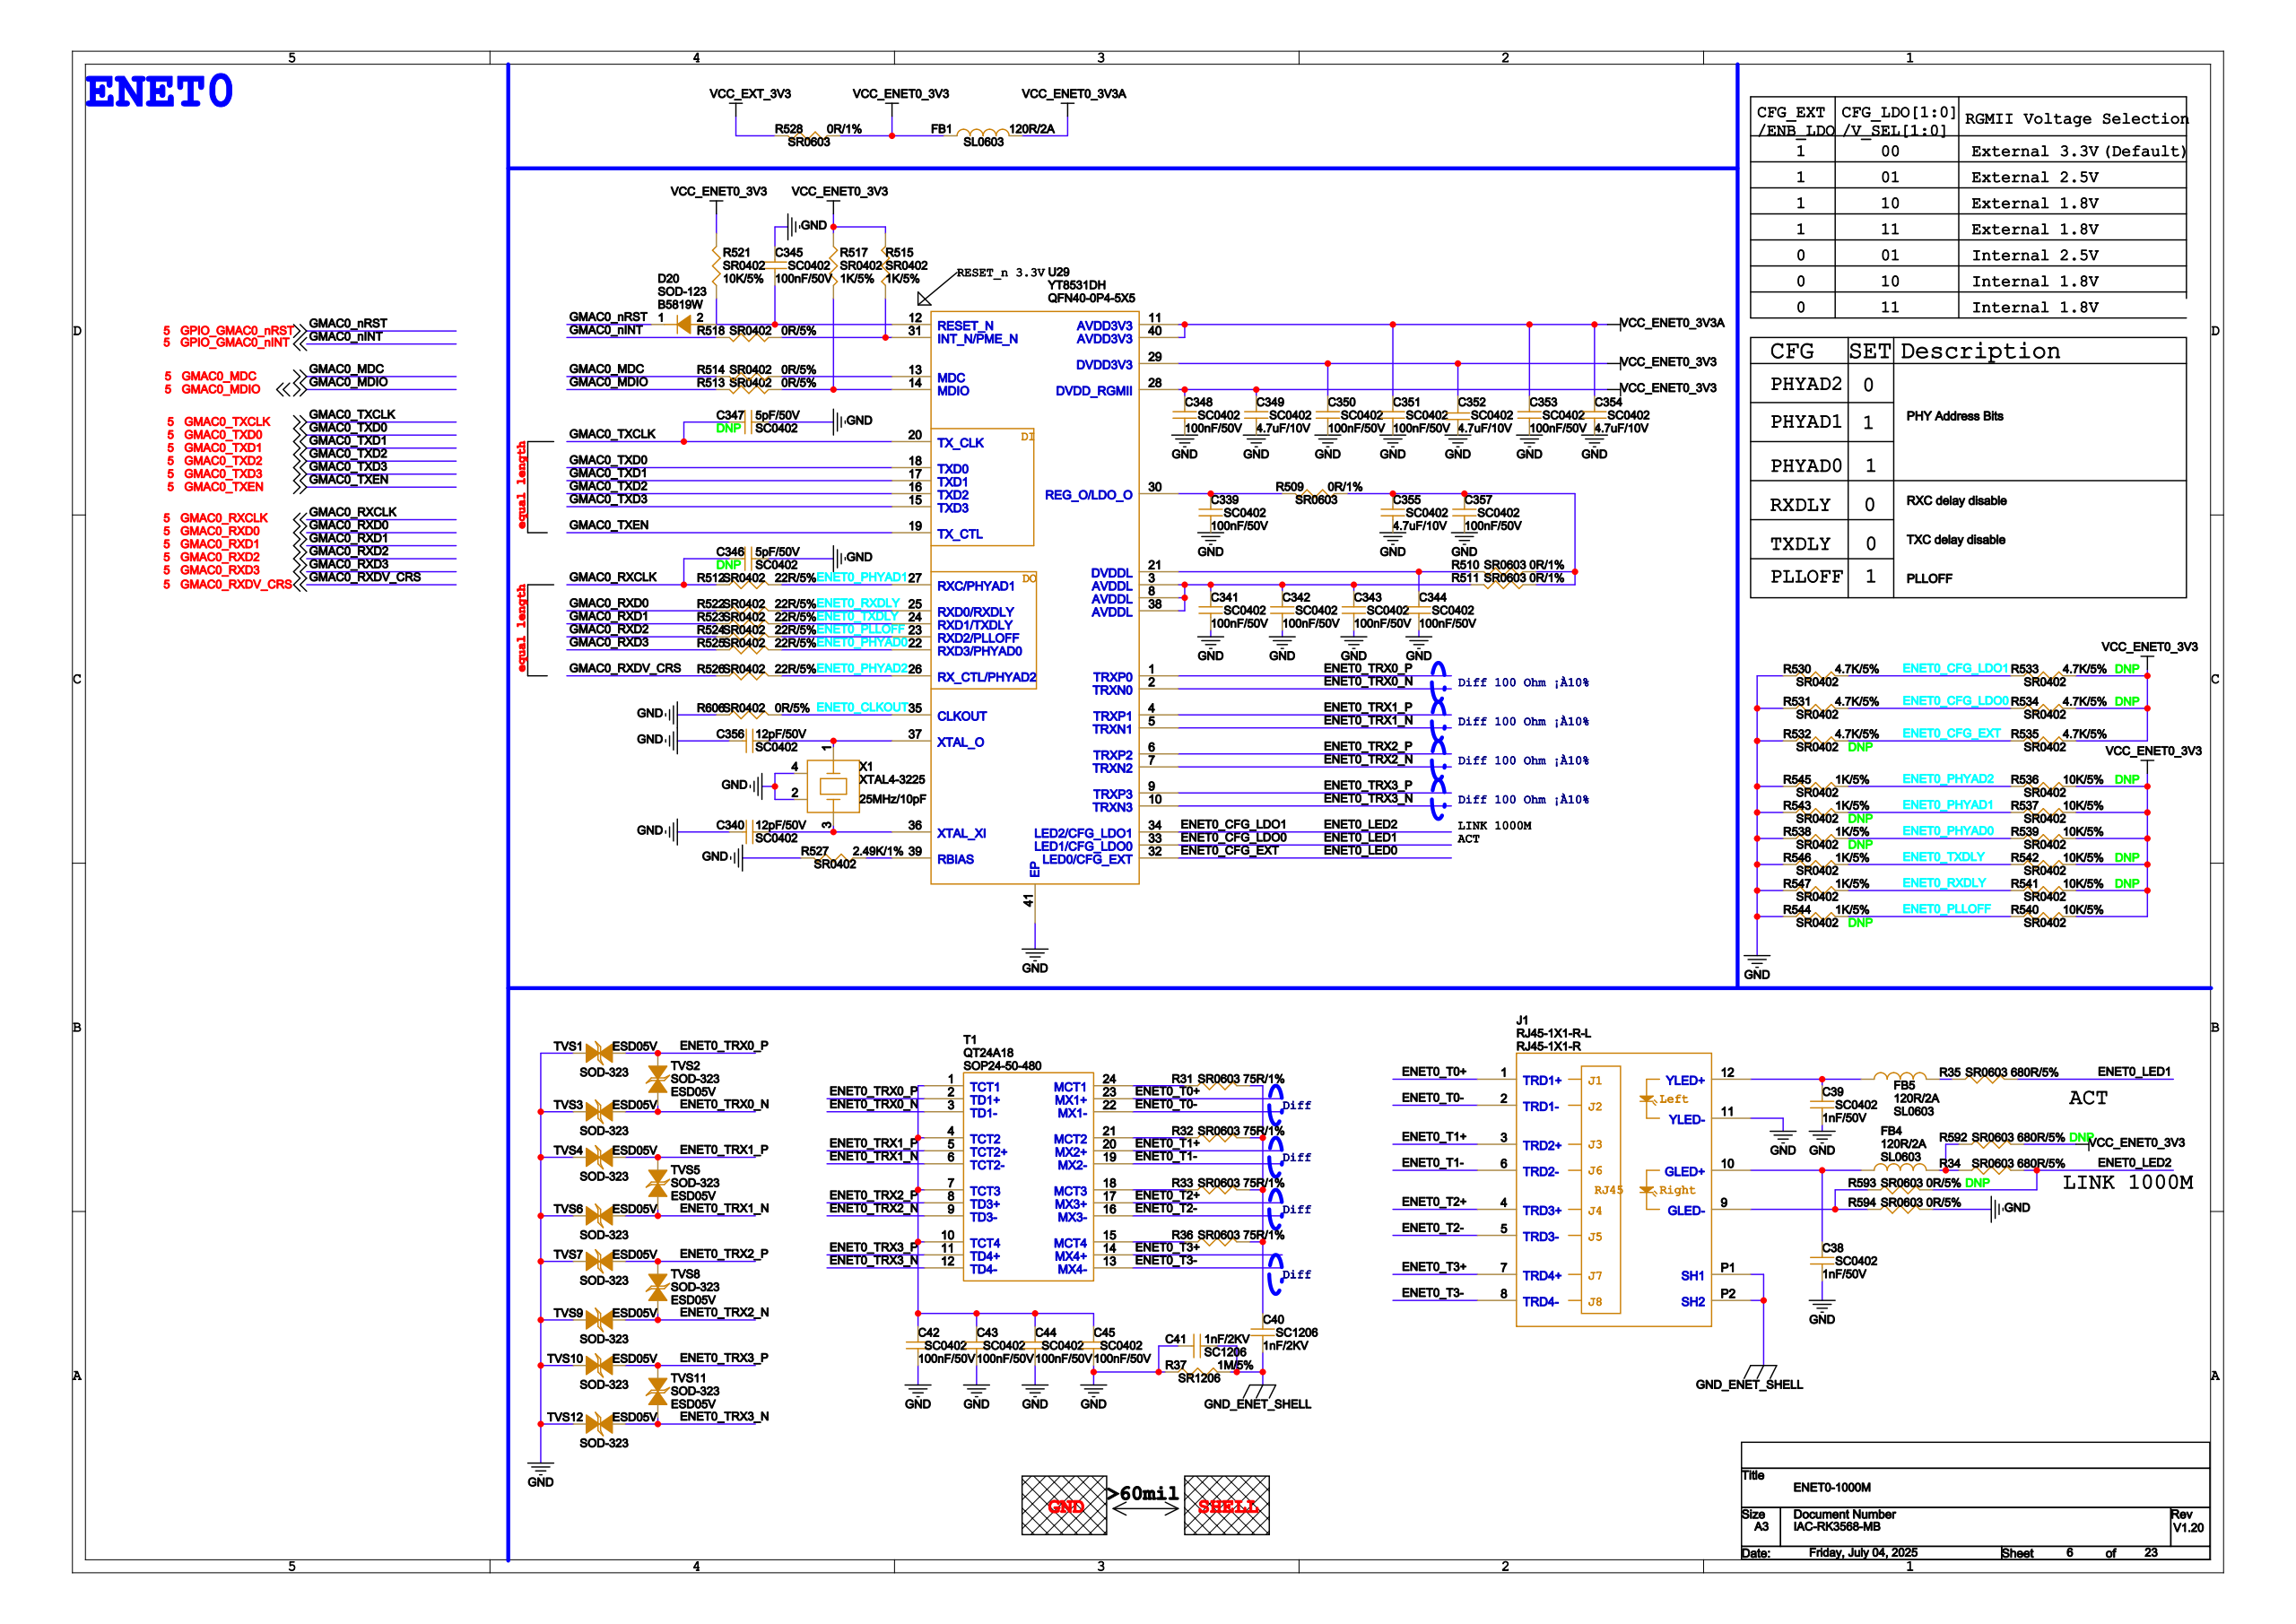Circuit board | Cadence Allegro | 1138 parts | 722 nets | one sheet of the schematic
Parts on this sheet (reference | value | footprint):
C38 | 1nF/50V | SC0402
C39 | 1nF/50V | SC0402
C40 | 1nF/2KV | SC1206
C41 | 1nF/2KV | SC1206
C339 | 100nF/50V | SC0402
C340 | 12pF/50V | SC0402
C341 | 100nF/50V | SC0402
C342 | 100nF/50V | SC0402
C343 | 100nF/50V | SC0402
C344 | 100nF/50V | SC0402
C345 | 100nF/50V | SC0402
C346 | 5pF/50V | SC0402
C347 | 5pF/50V | SC0402
C348 | 100nF/50V | SC0402
C349 | 4.7uF/10V | SC0402
C350 | 100nF/50V | SC0402
C351 | 100nF/50V | SC0402
C352 | 4.7uF/10V | SC0402
C353 | 100nF/50V | SC0402
C354 | 4.7uF/10V | SC0402
C355 | 4.7uF/10V | SC0402
C356 | 12pF/50V | SC0402
C357 | 100nF/50V | SC0402
D20 | B5819W | SOD-123
FB1 | 120R/2A | SL0603
FB4 | 120R/2A | SL0603
FB5 | 120R/2A | SL0603
J1 | RJ45-1X1-R | RJ45-1X1-R-L
J3 | PCIE52-X2-RS | PCIE52-X2-RS-1
J4 | M2-BKEY | M2-BKEY
R31 | 75R/1% | SR0603
R32 | 75R/1% | SR0603
R33 | 75R/1% | SR0603
R34 | 680R/5% | SR0603
R35 | 680R/5% | SR0603
R36 | 75R/1% | SR0603
R37 | 1M/5% | SR1206
R509 | 0R/1% | SR0603
R510 | 0R/1% | SR0603
R511 | 0R/1% | SR0603
R513 | 0R/5% | SR0402
R514 | 0R/5% | SR0402
R515 | 1K/5% | SR0402
R517 | 1K/5% | SR0402
R518 | 0R/5% | SR0402
R521 | 10K/5% | SR0402
R527 | 2.49K/1% | SR0402
R528 | 0R/1% | SR0603
R530 | 4.7K/5% | SR0402
R531 | 4.7K/5% | SR0402
R532 | 4.7K/5% | SR0402
R533 | 4.7K/5% | SR0402
R534 | 4.7K/5% | SR0402
R535 | 4.7K/5% | SR0402
R536 | 10K/5% | SR0402
R537 | 10K/5% | SR0402
R538 | 1K/5% | SR0402
R539 | 10K/5% | SR0402
R540 | 10K/5% | SR0402
R541 | 10K/5% | SR0402
R542 | 10K/5% | SR0402
R543 | 1K/5% | SR0402
R544 | 1K/5% | SR0402
R545 | 1K/5% | SR0402
R546 | 1K/5% | SR0402
R547 | 1K/5% | SR0402
R592 | 680R/5% | SR0603
R593 | 0R/5% | SR0603
R594 | 0R/5% | SR0603
T1 | QT24A18 | SOP24-50-480
TVS2 | ESD05V | SOD-323
TVS3 | ESD05V | SOD-323
TVS4 | ESD05V | SOD-323
TVS5 | ESD05V | SOD-323
TVS6 | ESD05V | SOD-323
TVS7 | ESD05V | SOD-323
TVS8 | ESD05V | SOD-323
TVS9 | ESD05V | SOD-323
TVS10 | ESD05V | SOD-323
TVS11 | ESD05V | SOD-323
TVS12 | ESD05V | SOD-323
U29 | YT8531DH | QFN40-0P4-5X5
X1 | 25MHz/10pF | XTAL4-3225
Nets of these parts (net: part-pin ...):
N5399426: C345-2 D20-2 R521-1 U29-12
GPIO_GMAC0_NRST: D20-1
VCC_EXT_3V3: R528-2
GND: C38-2 C39-2 C41-1 C339-2 C340-2 C341-2 C342-2 C343-2 C344-2 C345-1 C346-2 C347-2 C348-2 C349-2 C350-2 C351-2 C352-1 C353-2 C354-2 C355-2 C356-2 C357-2 J1-11 R37-1 R527-2 R530-1 R531-1 R532-1 R538-1 R543-1 R544-1 R545-1 R546-1 R547-1 R594-2 TVS3-1 TVS4-1 TVS6-1 TVS7-1 TVS9-1 TVS10-1 TVS12-1 X1-2 X1-4 J3-4 J3-9 J3-15 J3-18 J3-21 J3-26 J3-27 J3-29 J3-34 J3-35 J3-37 J3-40 J4-3 J4-5 J4-11 J4-27 J4-33 J4-39 U29-41
ENET0_TRX0_P: TVS2-2 T1-2 U29-1
ENET0_TRX3_P: TVS10-2 TVS11-2 T1-11 U29-9
ENET0_TRX3_N: TVS11-1 TVS12-2 T1-12 U29-10
ENET0_TRX0_N: TVS2-1 TVS3-2 T1-3 U29-2
ENET0_TRX1_P: TVS4-2 TVS5-2 T1-5 U29-4
ENET0_TRX1_N: TVS5-1 TVS6-2 T1-6 U29-5
ENET0_TRX2_P: TVS7-2 TVS8-2 T1-8 U29-6
ENET0_TRX2_N: TVS8-1 TVS9-2 T1-9 U29-7
N78733: C38-1 FB4-1 J1-10
N78487: J1-9 R593-1 R594-1
GND_ENET_SHELL: C40-2 C41-2 J1-P1 J1-P2 R37-2
ENET0_T0+: J1-1 T1-23
ENET0_T0-: J1-2 T1-22
ENET0_T1+: J1-3 T1-20
ENET0_T1-: J1-6 T1-19
ENET0_T2+: J1-4 T1-17
ENET0_T2-: J1-5 T1-16
ENET0_T3+: J1-7 T1-14
ENET0_T3-: J1-8 T1-13
N78531: C39-1 FB5-1 J1-12
N78681: C40-1 R31-2 R32-2 R33-2 R36-2
GMAC0_RXCLK: C346-1
GMAC0_TXCLK: C347-1 U29-20
N78791: FB4-2 R34-1 R592-1
ENET0_CFG_LDO1: R34-2 R530-2 R533-1 R593-2 U29-34
N78559: FB5-2 R35-1
ENET0_CFG_LDO0: R35-2 R531-2 R534-1 U29-33
VCC_ENET0_3V3: C348-1 C349-1 C350-1 C352-2 FB1-1 R515-2 R517-1 R521-2 R528-1 R533-2 R534-2 R535-2 R536-2 R537-2 R539-2 R540-1 R541-2 R542-2 R592-2 U29-28 U29-29
N78677: R31-1 T1-24
N78749: R32-1 T1-21
N78821: R33-1 T1-18
N78893: R36-1 T1-15
GMAC0_TXD0: U29-18
GMAC0_TXD1: U29-17
GMAC0_TXD2: U29-16
GMAC0_TXD3: U29-15
GMAC0_TXEN: U29-19
GMAC0_MDC: R514-2
GMAC0_MDIO: R513-2
GPIO_GMAC0_NINT: R518-2
N5399756: C339-1 R509-2 U29-30
N5400176: C341-1 C342-1 C343-1 R511-2 U29-3 U29-8 U29-38
N5400190: C344-1 R510-2 U29-21
VCC_ENET0_3V3A: C351-1 C353-1 C354-1 FB1-2 U29-11 U29-40
N5399696: C355-1 C357-1 R509-1 R510-1 R511-1
N5398966: C340-1 X1-3 U29-36
N5400472: C356-1 X1-1 U29-37
ENET0_PHYAD1: R537-1 R543-2 U29-27
ENET0_RXDLY: R541-1 R547-2 U29-25
ENET0_TXDLY: R542-1 R546-2 U29-24
ENET0_PLLOFF: R540-2 R544-2 U29-23
ENET0_PHYAD0: R538-2 R539-1 U29-22
ENET0_PHYAD2: R536-1 R545-2 U29-26
ENET0_CLKOUT: U29-35
N5399060: R513-1 R517-2 U29-14
N5399708: R514-1 U29-13
N5399158: R515-1 R518-1 U29-31
N5399124: R527-1 U29-39
ENET0_CFG_EXT: R532-2 R535-1 U29-32